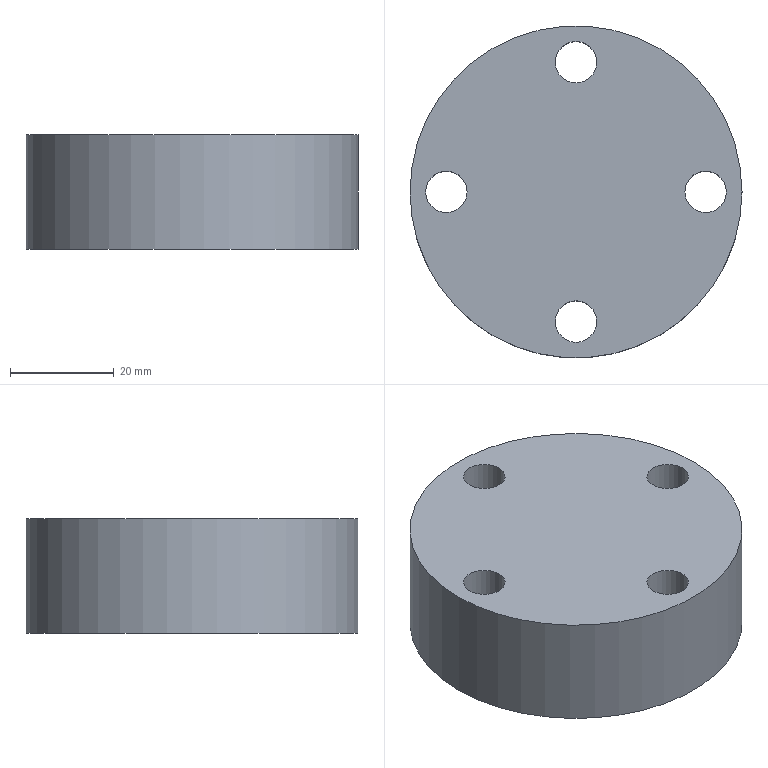Part | NX | 1 solid | 7 faces | box 64 x 64 x 22 mm | volume 66350 mm3 | cylinder 5 | plane 2 | commonest cylinder face diameters 8 x4 64 x1
STEP:
#1=CARTESIAN_POINT('',(0.,-29.,0.));
#2=VERTEX_POINT('',#1);
#3=CARTESIAN_POINT('',(0.,-25.,0.));
#4=DIRECTION('',(0.,0.,1.));
#5=DIRECTION('',(0.,-1.,0.));
#6=AXIS2_PLACEMENT_3D('',#3,#4,#5);
#7=CIRCLE('',#6,4.);
#8=EDGE_CURVE('',#2,#2,#7,.T.);
#9=ORIENTED_EDGE('',*,*,#8,.T.);
#10=EDGE_LOOP('',(#9));
#11=FACE_BOUND('',#10,.T.);
#12=CARTESIAN_POINT('',(0.,-29.,-22.));
#13=VERTEX_POINT('',#12);
#14=CARTESIAN_POINT('',(0.,-25.,-22.));
#15=DIRECTION('',(0.,0.,1.));
#16=DIRECTION('',(0.,-1.,0.));
#17=AXIS2_PLACEMENT_3D('',#14,#15,#16);
#18=CIRCLE('',#17,4.);
#19=EDGE_CURVE('',#13,#13,#18,.T.);
#20=ORIENTED_EDGE('',*,*,#19,.F.);
#21=EDGE_LOOP('',(#20));
#22=FACE_BOUND('',#21,.T.);
#23=CARTESIAN_POINT('',(0.,-25.,0.));
#24=DIRECTION('',(0.,0.,-1.));
#25=DIRECTION('',(-1.,0.,0.));
#26=AXIS2_PLACEMENT_3D('',#23,#24,#25);
#27=CYLINDRICAL_SURFACE('',#26,4.);
#28=ADVANCED_FACE('',(#11,#22),#27,.F.);
#29=CARTESIAN_POINT('',(0.,29.,0.));
#30=VERTEX_POINT('',#29);
#31=CARTESIAN_POINT('',(0.,25.,0.));
#32=DIRECTION('',(0.,0.,1.));
#33=DIRECTION('',(0.,1.,0.));
#34=AXIS2_PLACEMENT_3D('',#31,#32,#33);
#35=CIRCLE('',#34,4.);
#36=EDGE_CURVE('',#30,#30,#35,.T.);
#37=ORIENTED_EDGE('',*,*,#36,.T.);
#38=EDGE_LOOP('',(#37));
#39=FACE_BOUND('',#38,.T.);
#40=CARTESIAN_POINT('',(0.,29.,-22.));
#41=VERTEX_POINT('',#40);
#42=CARTESIAN_POINT('',(0.,25.,-22.));
#43=DIRECTION('',(0.,0.,1.));
#44=DIRECTION('',(0.,1.,0.));
#45=AXIS2_PLACEMENT_3D('',#42,#43,#44);
#46=CIRCLE('',#45,4.);
#47=EDGE_CURVE('',#41,#41,#46,.T.);
#48=ORIENTED_EDGE('',*,*,#47,.F.);
#49=EDGE_LOOP('',(#48));
#50=FACE_BOUND('',#49,.T.);
#51=CARTESIAN_POINT('',(0.,25.,0.));
#52=DIRECTION('',(0.,0.,-1.));
#53=DIRECTION('',(-1.,0.,0.));
#54=AXIS2_PLACEMENT_3D('',#51,#52,#53);
#55=CYLINDRICAL_SURFACE('',#54,4.);
#56=ADVANCED_FACE('',(#39,#50),#55,.F.);
#57=CARTESIAN_POINT('',(29.,0.,0.));
#58=VERTEX_POINT('',#57);
#59=CARTESIAN_POINT('',(25.,0.,0.));
#60=DIRECTION('',(0.,0.,1.));
#61=DIRECTION('',(1.,0.,0.));
#62=AXIS2_PLACEMENT_3D('',#59,#60,#61);
#63=CIRCLE('',#62,4.);
#64=EDGE_CURVE('',#58,#58,#63,.T.);
#65=ORIENTED_EDGE('',*,*,#64,.T.);
#66=EDGE_LOOP('',(#65));
#67=FACE_BOUND('',#66,.T.);
#68=CARTESIAN_POINT('',(29.,0.,-22.));
#69=VERTEX_POINT('',#68);
#70=CARTESIAN_POINT('',(25.,0.,-22.));
#71=DIRECTION('',(0.,0.,1.));
#72=DIRECTION('',(1.,0.,0.));
#73=AXIS2_PLACEMENT_3D('',#70,#71,#72);
#74=CIRCLE('',#73,4.);
#75=EDGE_CURVE('',#69,#69,#74,.T.);
#76=ORIENTED_EDGE('',*,*,#75,.F.);
#77=EDGE_LOOP('',(#76));
#78=FACE_BOUND('',#77,.T.);
#79=CARTESIAN_POINT('',(25.,0.,0.));
#80=DIRECTION('',(0.,0.,-1.));
#81=DIRECTION('',(-1.,0.,0.));
#82=AXIS2_PLACEMENT_3D('',#79,#80,#81);
#83=CYLINDRICAL_SURFACE('',#82,4.);
#84=ADVANCED_FACE('',(#67,#78),#83,.F.);
#85=CARTESIAN_POINT('',(32.,0.,0.));
#86=VERTEX_POINT('',#85);
#87=CARTESIAN_POINT('',(0.,0.,0.));
#88=DIRECTION('',(0.,0.,-1.));
#89=DIRECTION('',(1.,0.,0.));
#90=AXIS2_PLACEMENT_3D('',#87,#88,#89);
#91=CIRCLE('',#90,32.);
#92=EDGE_CURVE('',#86,#86,#91,.T.);
#93=ORIENTED_EDGE('',*,*,#92,.T.);
#94=EDGE_LOOP('',(#93));
#95=FACE_BOUND('',#94,.T.);
#96=CARTESIAN_POINT('',(32.,0.,-22.));
#97=VERTEX_POINT('',#96);
#98=CARTESIAN_POINT('',(0.,0.,-22.));
#99=DIRECTION('',(0.,0.,-1.));
#100=DIRECTION('',(1.,0.,0.));
#101=AXIS2_PLACEMENT_3D('',#98,#99,#100);
#102=CIRCLE('',#101,32.);
#103=EDGE_CURVE('',#97,#97,#102,.T.);
#104=ORIENTED_EDGE('',*,*,#103,.F.);
#105=EDGE_LOOP('',(#104));
#106=FACE_BOUND('',#105,.T.);
#107=CARTESIAN_POINT('',(0.,0.,0.));
#108=DIRECTION('',(0.,0.,-1.));
#109=DIRECTION('',(-1.,0.,0.));
#110=AXIS2_PLACEMENT_3D('',#107,#108,#109);
#111=CYLINDRICAL_SURFACE('',#110,32.);
#112=ADVANCED_FACE('',(#95,#106),#111,.T.);
#113=CARTESIAN_POINT('',(-29.,0.,0.));
#114=VERTEX_POINT('',#113);
#115=CARTESIAN_POINT('',(-25.,0.,0.));
#116=DIRECTION('',(0.,0.,1.));
#117=DIRECTION('',(-1.,0.,0.));
#118=AXIS2_PLACEMENT_3D('',#115,#116,#117);
#119=CIRCLE('',#118,4.);
#120=EDGE_CURVE('',#114,#114,#119,.T.);
#121=ORIENTED_EDGE('',*,*,#120,.T.);
#122=EDGE_LOOP('',(#121));
#123=FACE_BOUND('',#122,.T.);
#124=CARTESIAN_POINT('',(-29.,0.,-22.));
#125=VERTEX_POINT('',#124);
#126=CARTESIAN_POINT('',(-25.,0.,-22.));
#127=DIRECTION('',(0.,0.,1.));
#128=DIRECTION('',(-1.,0.,0.));
#129=AXIS2_PLACEMENT_3D('',#126,#127,#128);
#130=CIRCLE('',#129,4.);
#131=EDGE_CURVE('',#125,#125,#130,.T.);
#132=ORIENTED_EDGE('',*,*,#131,.F.);
#133=EDGE_LOOP('',(#132));
#134=FACE_BOUND('',#133,.T.);
#135=CARTESIAN_POINT('',(-25.,0.,0.));
#136=DIRECTION('',(0.,0.,-1.));
#137=DIRECTION('',(-1.,0.,0.));
#138=AXIS2_PLACEMENT_3D('',#135,#136,#137);
#139=CYLINDRICAL_SURFACE('',#138,4.);
#140=ADVANCED_FACE('',(#123,#134),#139,.F.);
#141=ORIENTED_EDGE('',*,*,#92,.F.);
#142=EDGE_LOOP('',(#141));
#143=FACE_BOUND('',#142,.T.);
#144=ORIENTED_EDGE('',*,*,#64,.F.);
#145=EDGE_LOOP('',(#144));
#146=FACE_BOUND('',#145,.T.);
#147=ORIENTED_EDGE('',*,*,#36,.F.);
#148=EDGE_LOOP('',(#147));
#149=FACE_BOUND('',#148,.T.);
#150=ORIENTED_EDGE('',*,*,#8,.F.);
#151=EDGE_LOOP('',(#150));
#152=FACE_BOUND('',#151,.T.);
#153=ORIENTED_EDGE('',*,*,#120,.F.);
#154=EDGE_LOOP('',(#153));
#155=FACE_BOUND('',#154,.T.);
#156=CARTESIAN_POINT('',(12.5,0.,0.));
#157=DIRECTION('',(0.,0.,-1.));
#158=DIRECTION('',(-1.,0.,0.));
#159=AXIS2_PLACEMENT_3D('',#156,#157,#158);
#160=PLANE('',#159);
#161=ADVANCED_FACE('',(#143,#146,#149,#152,#155),#160,.F.);
#162=ORIENTED_EDGE('',*,*,#103,.T.);
#163=EDGE_LOOP('',(#162));
#164=FACE_BOUND('',#163,.T.);
#165=ORIENTED_EDGE('',*,*,#75,.T.);
#166=EDGE_LOOP('',(#165));
#167=FACE_BOUND('',#166,.T.);
#168=ORIENTED_EDGE('',*,*,#47,.T.);
#169=EDGE_LOOP('',(#168));
#170=FACE_BOUND('',#169,.T.);
#171=ORIENTED_EDGE('',*,*,#19,.T.);
#172=EDGE_LOOP('',(#171));
#173=FACE_BOUND('',#172,.T.);
#174=ORIENTED_EDGE('',*,*,#131,.T.);
#175=EDGE_LOOP('',(#174));
#176=FACE_BOUND('',#175,.T.);
#177=CARTESIAN_POINT('',(12.5,0.,-22.));
#178=DIRECTION('',(0.,0.,-1.));
#179=DIRECTION('',(-1.,0.,0.));
#180=AXIS2_PLACEMENT_3D('',#177,#178,#179);
#181=PLANE('',#180);
#182=ADVANCED_FACE('',(#164,#167,#170,#173,#176),#181,.T.);
#183=CLOSED_SHELL('',(#28,#56,#84,#112,#140,#161,#182));
#184=MANIFOLD_SOLID_BREP('',#183);
#185=(LENGTH_UNIT()NAMED_UNIT(*)SI_UNIT(.MILLI.,.METRE.));
#186=UNCERTAINTY_MEASURE_WITH_UNIT(LENGTH_MEASURE(0.00001),#185,'','');
#187=(NAMED_UNIT(*)PLANE_ANGLE_UNIT()SI_UNIT($,.RADIAN.));
#188=(NAMED_UNIT(*)SI_UNIT($,.STERADIAN.)SOLID_ANGLE_UNIT());
#189=(GEOMETRIC_REPRESENTATION_CONTEXT(3)GLOBAL_UNCERTAINTY_ASSIGNED_CONTEXT((#186))GLOBAL_UNIT_ASSIGNED_CONTEXT((#185,#187,#188))REPRESENTATION_CONTEXT('',''));
#190=ADVANCED_BREP_SHAPE_REPRESENTATION('',(#184),#189);